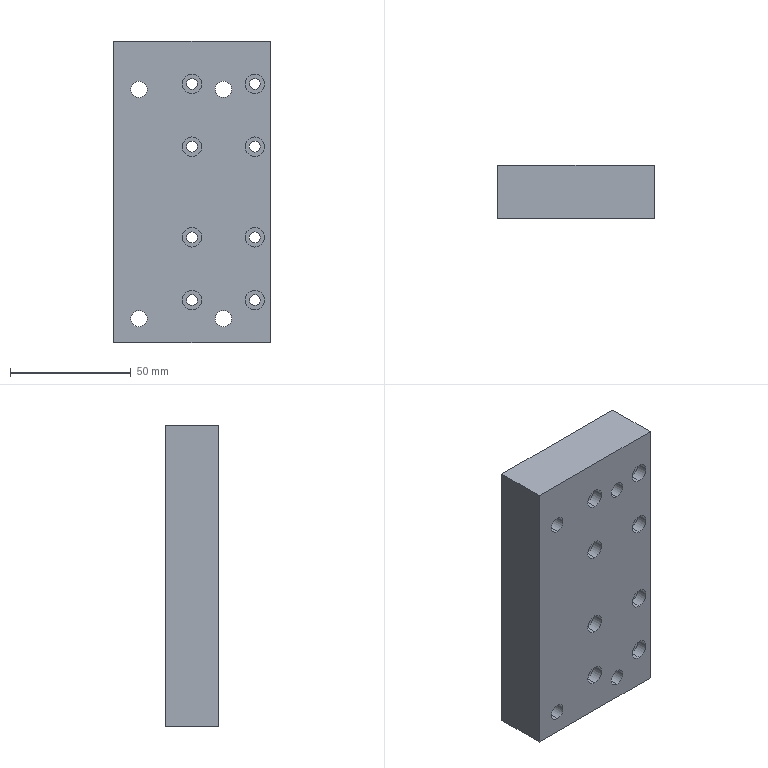Part | STEP file | X77-07005 | 1 solid | 54 faces | box 65 x 22 x 125 mm | volume 171490 mm3 | cylinder 40 | plane 14 | commonest cylinder face diameters 4.5 x16 8 x16 6.8 x8